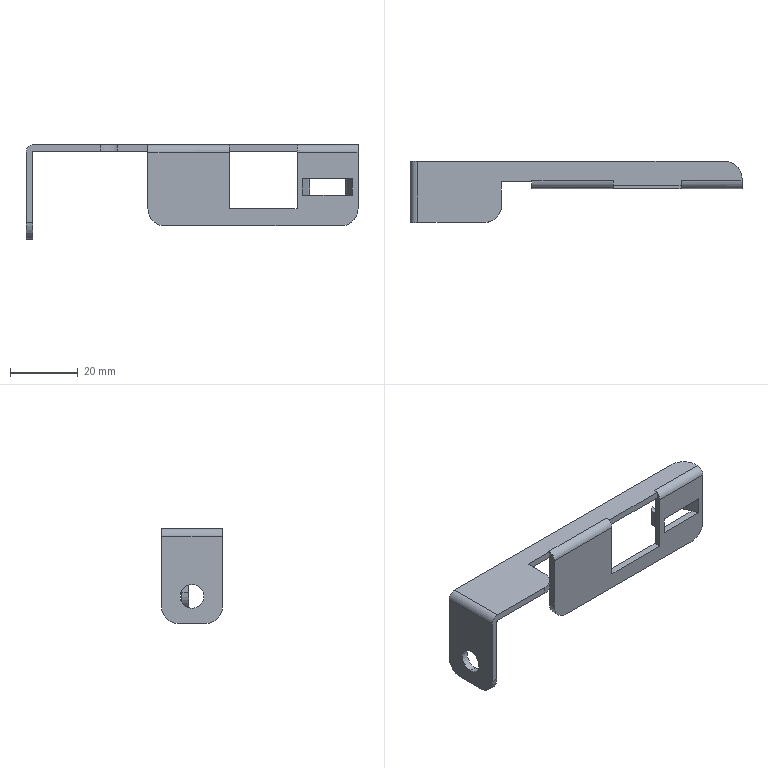Part | STEP file | Upper pull rod (lower door) | 1 solid | 51 faces | box 98 x 18 x 28 mm | volume 4727 mm3 | plane 33 | cylinder 18 | commonest cylinder face diameters 10 x6 0.6 x3 4.6 x3 4.62 x2 7 x2 8.62 x2